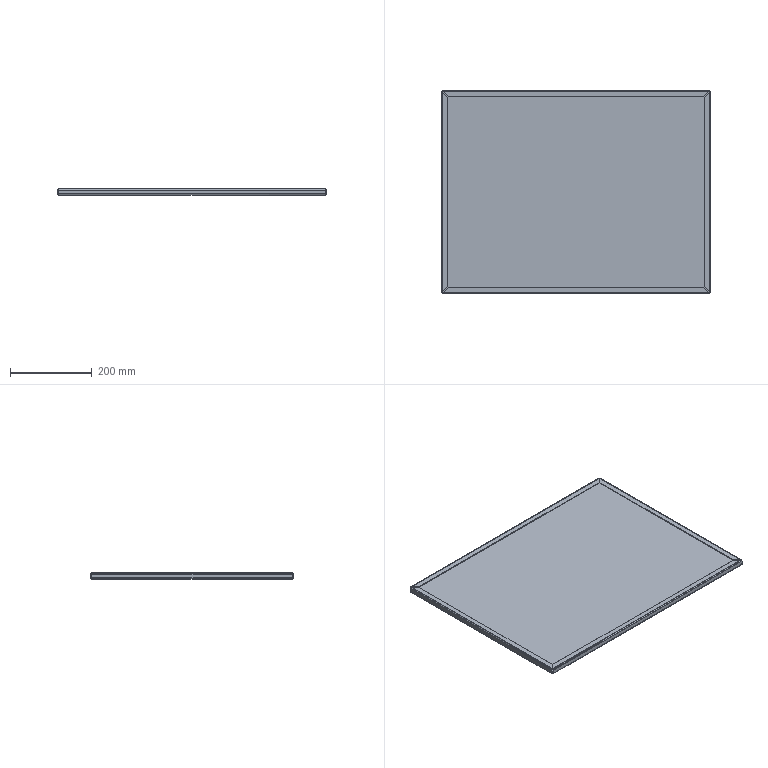Part | STEP file | Distribution box door SGN-1-12-04 | 1 solid | 70 faces | box 656 x 494 x 15 mm | volume 458651 mm3 | plane 38 | spline 16 | cylinder 16 | commonest cylinder face diameters 3 x8 5.4 x8